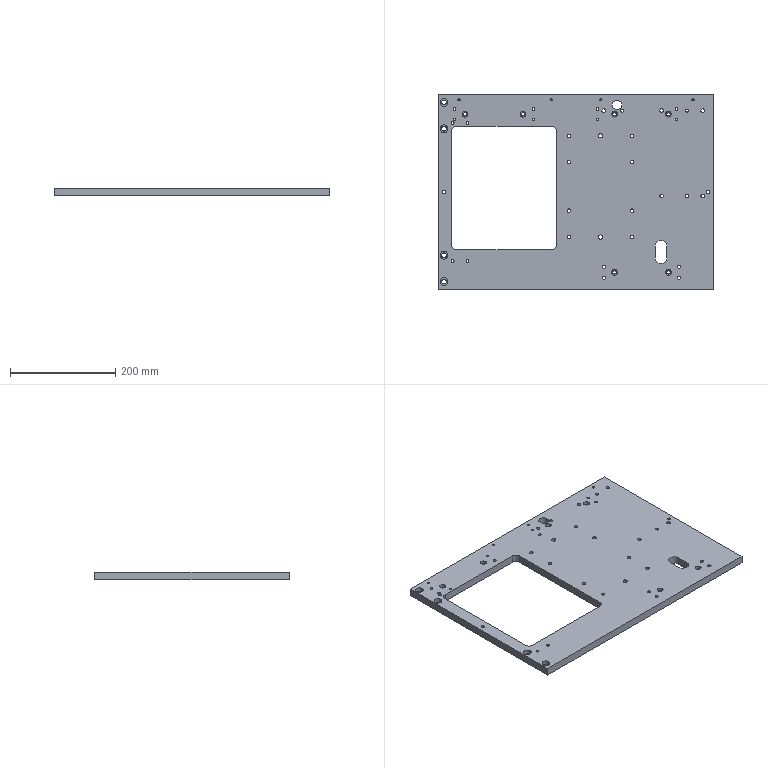Part | 1 solid | 182 faces | box 521 x 370 x 15 mm | volume 2140262 mm3 | cylinder 136 | cone 24 | plane 22 | commonest cylinder face diameters 5 x32 6.8 x26 6 x18 6.6 x12 11 x12 3.3 x8